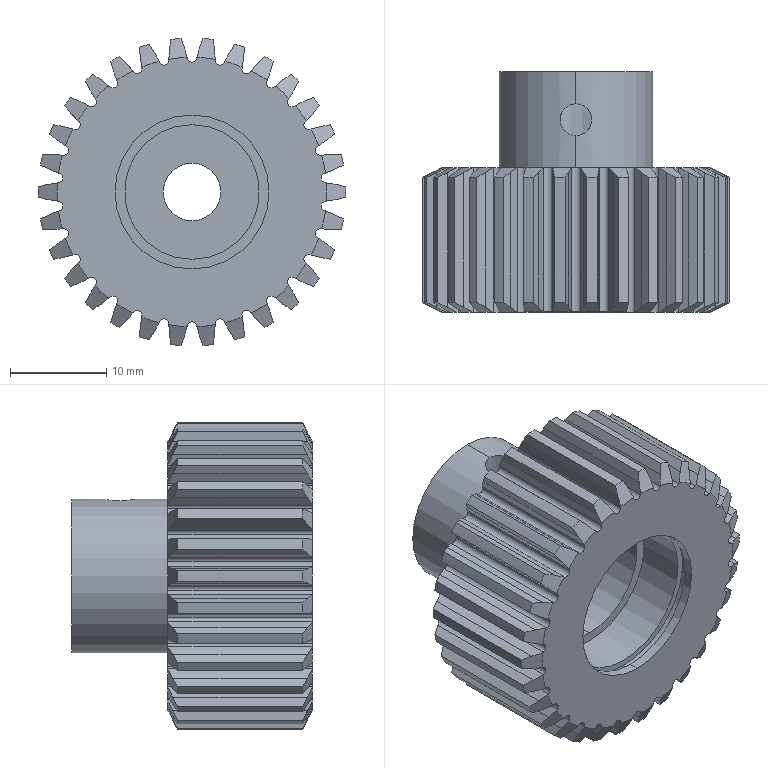Part | STEP file | 04-04 Suction gear | 1 solid | 278 faces | box 32 x 25 x 31.918 mm | volume 9255 mm3 | plane 128 | cylinder 89 | cone 61 | commonest cylinder face diameters 1 x42 32 x31 16 x6 3.3 x2 6 x2 10 x2